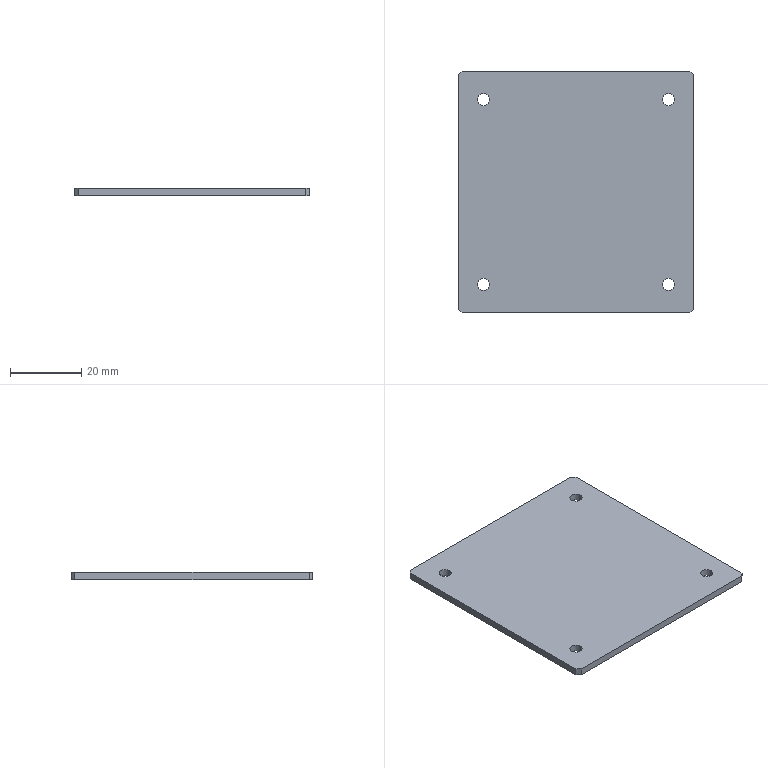Part | SolidWorks | features BaseBody 1 | 1 solid | 18 faces | box 66 x 68 x 2 mm | volume 8899 mm3 | plane 10 | cylinder 8 | commonest cylinder face diameters 3.4 x8
STEP:
#1=CARTESIAN_POINT('',(24.3,-26.,0.));
#2=VERTEX_POINT('',#1);
#3=CARTESIAN_POINT('',(27.7,-26.,0.));
#4=VERTEX_POINT('',#3);
#5=CARTESIAN_POINT('',(26.,-26.,0.));
#6=DIRECTION('',(0.,0.,1.));
#7=DIRECTION('',(1.,0.,0.));
#8=AXIS2_PLACEMENT_3D('',#5,#6,#7);
#9=CIRCLE('',#8,1.7);
#10=EDGE_CURVE('',#2,#4,#9,.T.);
#11=ORIENTED_EDGE('',*,*,#10,.F.);
#12=CARTESIAN_POINT('',(24.3,-26.,2.));
#13=VERTEX_POINT('',#12);
#14=CARTESIAN_POINT('',(24.3,-26.,2.));
#15=DIRECTION('',(0.,0.,1.));
#16=VECTOR('',#15,1000.);
#17=LINE('',#14,#16);
#18=EDGE_CURVE('',#2,#13,#17,.T.);
#19=ORIENTED_EDGE('',*,*,#18,.T.);
#20=CARTESIAN_POINT('',(27.7,-26.,2.));
#21=VERTEX_POINT('',#20);
#22=CARTESIAN_POINT('',(26.,-26.,2.));
#23=DIRECTION('',(0.,0.,-1.));
#24=DIRECTION('',(1.,0.,0.));
#25=AXIS2_PLACEMENT_3D('',#22,#23,#24);
#26=CIRCLE('',#25,1.7);
#27=EDGE_CURVE('',#21,#13,#26,.T.);
#28=ORIENTED_EDGE('',*,*,#27,.F.);
#29=CARTESIAN_POINT('',(27.7,-26.,2.));
#30=DIRECTION('',(0.,0.,1.));
#31=VECTOR('',#30,1000.);
#32=LINE('',#29,#31);
#33=EDGE_CURVE('',#4,#21,#32,.T.);
#34=ORIENTED_EDGE('',*,*,#33,.F.);
#35=EDGE_LOOP('',(#11,#19,#28,#34));
#36=FACE_OUTER_BOUND('',#35,.T.);
#37=CARTESIAN_POINT('',(26.,-26.,2.));
#38=DIRECTION('',(0.,0.,1.));
#39=DIRECTION('',(1.,0.,0.));
#40=AXIS2_PLACEMENT_3D('',#37,#38,#39);
#41=CYLINDRICAL_SURFACE('',#40,1.7);
#42=ADVANCED_FACE('',(#36),#41,.F.);
#43=CARTESIAN_POINT('',(24.3,26.,0.));
#44=VERTEX_POINT('',#43);
#45=CARTESIAN_POINT('',(27.7,26.,0.));
#46=VERTEX_POINT('',#45);
#47=CARTESIAN_POINT('',(26.,26.,0.));
#48=DIRECTION('',(0.,0.,1.));
#49=DIRECTION('',(1.,0.,0.));
#50=AXIS2_PLACEMENT_3D('',#47,#48,#49);
#51=CIRCLE('',#50,1.7);
#52=EDGE_CURVE('',#44,#46,#51,.T.);
#53=ORIENTED_EDGE('',*,*,#52,.F.);
#54=CARTESIAN_POINT('',(24.3,26.,2.));
#55=VERTEX_POINT('',#54);
#56=CARTESIAN_POINT('',(24.3,26.,2.));
#57=DIRECTION('',(0.,0.,1.));
#58=VECTOR('',#57,1000.);
#59=LINE('',#56,#58);
#60=EDGE_CURVE('',#44,#55,#59,.T.);
#61=ORIENTED_EDGE('',*,*,#60,.T.);
#62=CARTESIAN_POINT('',(27.7,26.,2.));
#63=VERTEX_POINT('',#62);
#64=CARTESIAN_POINT('',(26.,26.,2.));
#65=DIRECTION('',(0.,0.,-1.));
#66=DIRECTION('',(1.,0.,0.));
#67=AXIS2_PLACEMENT_3D('',#64,#65,#66);
#68=CIRCLE('',#67,1.7);
#69=EDGE_CURVE('',#63,#55,#68,.T.);
#70=ORIENTED_EDGE('',*,*,#69,.F.);
#71=CARTESIAN_POINT('',(27.7,26.,2.));
#72=DIRECTION('',(0.,0.,1.));
#73=VECTOR('',#72,1000.);
#74=LINE('',#71,#73);
#75=EDGE_CURVE('',#46,#63,#74,.T.);
#76=ORIENTED_EDGE('',*,*,#75,.F.);
#77=EDGE_LOOP('',(#53,#61,#70,#76));
#78=FACE_OUTER_BOUND('',#77,.T.);
#79=CARTESIAN_POINT('',(26.,26.,2.));
#80=DIRECTION('',(0.,0.,1.));
#81=DIRECTION('',(1.,0.,0.));
#82=AXIS2_PLACEMENT_3D('',#79,#80,#81);
#83=CYLINDRICAL_SURFACE('',#82,1.7);
#84=ADVANCED_FACE('',(#78),#83,.F.);
#85=CARTESIAN_POINT('',(-27.7,26.,0.));
#86=VERTEX_POINT('',#85);
#87=CARTESIAN_POINT('',(-24.3,26.,0.));
#88=VERTEX_POINT('',#87);
#89=CARTESIAN_POINT('',(-26.,26.,0.));
#90=DIRECTION('',(0.,0.,1.));
#91=DIRECTION('',(1.,0.,0.));
#92=AXIS2_PLACEMENT_3D('',#89,#90,#91);
#93=CIRCLE('',#92,1.7);
#94=EDGE_CURVE('',#86,#88,#93,.T.);
#95=ORIENTED_EDGE('',*,*,#94,.F.);
#96=CARTESIAN_POINT('',(-27.7,26.,2.));
#97=VERTEX_POINT('',#96);
#98=CARTESIAN_POINT('',(-27.7,26.,2.));
#99=DIRECTION('',(0.,0.,1.));
#100=VECTOR('',#99,1000.);
#101=LINE('',#98,#100);
#102=EDGE_CURVE('',#86,#97,#101,.T.);
#103=ORIENTED_EDGE('',*,*,#102,.T.);
#104=CARTESIAN_POINT('',(-24.3,26.,2.));
#105=VERTEX_POINT('',#104);
#106=CARTESIAN_POINT('',(-26.,26.,2.));
#107=DIRECTION('',(0.,0.,-1.));
#108=DIRECTION('',(1.,0.,0.));
#109=AXIS2_PLACEMENT_3D('',#106,#107,#108);
#110=CIRCLE('',#109,1.7);
#111=EDGE_CURVE('',#105,#97,#110,.T.);
#112=ORIENTED_EDGE('',*,*,#111,.F.);
#113=CARTESIAN_POINT('',(-24.3,26.,2.));
#114=DIRECTION('',(0.,0.,1.));
#115=VECTOR('',#114,1000.);
#116=LINE('',#113,#115);
#117=EDGE_CURVE('',#88,#105,#116,.T.);
#118=ORIENTED_EDGE('',*,*,#117,.F.);
#119=EDGE_LOOP('',(#95,#103,#112,#118));
#120=FACE_OUTER_BOUND('',#119,.T.);
#121=CARTESIAN_POINT('',(-26.,26.,2.));
#122=DIRECTION('',(0.,0.,1.));
#123=DIRECTION('',(1.,0.,0.));
#124=AXIS2_PLACEMENT_3D('',#121,#122,#123);
#125=CYLINDRICAL_SURFACE('',#124,1.7);
#126=ADVANCED_FACE('',(#120),#125,.F.);
#127=CARTESIAN_POINT('',(-27.7,-26.,0.));
#128=VERTEX_POINT('',#127);
#129=CARTESIAN_POINT('',(-24.3,-26.,0.));
#130=VERTEX_POINT('',#129);
#131=CARTESIAN_POINT('',(-26.,-26.,0.));
#132=DIRECTION('',(0.,0.,1.));
#133=DIRECTION('',(1.,0.,0.));
#134=AXIS2_PLACEMENT_3D('',#131,#132,#133);
#135=CIRCLE('',#134,1.7);
#136=EDGE_CURVE('',#128,#130,#135,.T.);
#137=ORIENTED_EDGE('',*,*,#136,.F.);
#138=CARTESIAN_POINT('',(-27.7,-26.,2.));
#139=VERTEX_POINT('',#138);
#140=CARTESIAN_POINT('',(-27.7,-26.,2.));
#141=DIRECTION('',(0.,0.,1.));
#142=VECTOR('',#141,1000.);
#143=LINE('',#140,#142);
#144=EDGE_CURVE('',#128,#139,#143,.T.);
#145=ORIENTED_EDGE('',*,*,#144,.T.);
#146=CARTESIAN_POINT('',(-24.3,-26.,2.));
#147=VERTEX_POINT('',#146);
#148=CARTESIAN_POINT('',(-26.,-26.,2.));
#149=DIRECTION('',(0.,0.,-1.));
#150=DIRECTION('',(1.,0.,0.));
#151=AXIS2_PLACEMENT_3D('',#148,#149,#150);
#152=CIRCLE('',#151,1.7);
#153=EDGE_CURVE('',#147,#139,#152,.T.);
#154=ORIENTED_EDGE('',*,*,#153,.F.);
#155=CARTESIAN_POINT('',(-24.3,-26.,2.));
#156=DIRECTION('',(0.,0.,1.));
#157=VECTOR('',#156,1000.);
#158=LINE('',#155,#157);
#159=EDGE_CURVE('',#130,#147,#158,.T.);
#160=ORIENTED_EDGE('',*,*,#159,.F.);
#161=EDGE_LOOP('',(#137,#145,#154,#160));
#162=FACE_OUTER_BOUND('',#161,.T.);
#163=CARTESIAN_POINT('',(-26.,-26.,2.));
#164=DIRECTION('',(0.,0.,1.));
#165=DIRECTION('',(1.,0.,0.));
#166=AXIS2_PLACEMENT_3D('',#163,#164,#165);
#167=CYLINDRICAL_SURFACE('',#166,1.7);
#168=ADVANCED_FACE('',(#162),#167,.F.);
#169=CARTESIAN_POINT('',(-33.,33.,2.));
#170=VERTEX_POINT('',#169);
#171=CARTESIAN_POINT('',(-33.,-33.,2.));
#172=VERTEX_POINT('',#171);
#173=CARTESIAN_POINT('',(-33.,0.,2.));
#174=DIRECTION('',(0.,-1.,0.));
#175=VECTOR('',#174,1000.);
#176=LINE('',#173,#175);
#177=EDGE_CURVE('',#170,#172,#176,.T.);
#178=ORIENTED_EDGE('',*,*,#177,.T.);
#179=CARTESIAN_POINT('',(-32.,-34.,2.));
#180=VERTEX_POINT('',#179);
#181=CARTESIAN_POINT('',(-32.,-34.,2.));
#182=DIRECTION('',(0.7071,-0.7071,0.));
#183=VECTOR('',#182,1000.);
#184=LINE('',#181,#183);
#185=EDGE_CURVE('',#172,#180,#184,.T.);
#186=ORIENTED_EDGE('',*,*,#185,.T.);
#187=CARTESIAN_POINT('',(32.,-34.,2.));
#188=VERTEX_POINT('',#187);
#189=CARTESIAN_POINT('',(0.,-34.,2.));
#190=DIRECTION('',(1.,0.,0.));
#191=VECTOR('',#190,1000.);
#192=LINE('',#189,#191);
#193=EDGE_CURVE('',#180,#188,#192,.T.);
#194=ORIENTED_EDGE('',*,*,#193,.T.);
#195=CARTESIAN_POINT('',(33.,-33.,2.));
#196=VERTEX_POINT('',#195);
#197=CARTESIAN_POINT('',(33.,-33.,2.));
#198=DIRECTION('',(0.7071,0.7071,0.));
#199=VECTOR('',#198,1000.);
#200=LINE('',#197,#199);
#201=EDGE_CURVE('',#188,#196,#200,.T.);
#202=ORIENTED_EDGE('',*,*,#201,.T.);
#203=CARTESIAN_POINT('',(33.,33.,2.));
#204=VERTEX_POINT('',#203);
#205=CARTESIAN_POINT('',(33.,0.,2.));
#206=DIRECTION('',(0.,1.,0.));
#207=VECTOR('',#206,1000.);
#208=LINE('',#205,#207);
#209=EDGE_CURVE('',#196,#204,#208,.T.);
#210=ORIENTED_EDGE('',*,*,#209,.T.);
#211=CARTESIAN_POINT('',(32.,34.,2.));
#212=VERTEX_POINT('',#211);
#213=CARTESIAN_POINT('',(32.,34.,2.));
#214=DIRECTION('',(-0.7071,0.7071,0.));
#215=VECTOR('',#214,1000.);
#216=LINE('',#213,#215);
#217=EDGE_CURVE('',#204,#212,#216,.T.);
#218=ORIENTED_EDGE('',*,*,#217,.T.);
#219=CARTESIAN_POINT('',(-32.,34.,2.));
#220=VERTEX_POINT('',#219);
#221=CARTESIAN_POINT('',(0.,34.,2.));
#222=DIRECTION('',(-1.,0.,0.));
#223=VECTOR('',#222,1000.);
#224=LINE('',#221,#223);
#225=EDGE_CURVE('',#212,#220,#224,.T.);
#226=ORIENTED_EDGE('',*,*,#225,.T.);
#227=CARTESIAN_POINT('',(-33.,33.,2.));
#228=DIRECTION('',(-0.7071,-0.7071,0.));
#229=VECTOR('',#228,1000.);
#230=LINE('',#227,#229);
#231=EDGE_CURVE('',#220,#170,#230,.T.);
#232=ORIENTED_EDGE('',*,*,#231,.T.);
#233=EDGE_LOOP('',(#178,#186,#194,#202,#210,#218,#226,#232));
#234=FACE_OUTER_BOUND('',#233,.T.);
#235=ORIENTED_EDGE('',*,*,#27,.T.);
#236=CARTESIAN_POINT('',(26.,-26.,2.));
#237=DIRECTION('',(0.,0.,-1.));
#238=DIRECTION('',(1.,0.,0.));
#239=AXIS2_PLACEMENT_3D('',#236,#237,#238);
#240=CIRCLE('',#239,1.7);
#241=EDGE_CURVE('',#13,#21,#240,.T.);
#242=ORIENTED_EDGE('',*,*,#241,.T.);
#243=EDGE_LOOP('',(#235,#242));
#244=FACE_BOUND('',#243,.T.);
#245=ORIENTED_EDGE('',*,*,#69,.T.);
#246=CARTESIAN_POINT('',(26.,26.,2.));
#247=DIRECTION('',(0.,0.,-1.));
#248=DIRECTION('',(1.,0.,0.));
#249=AXIS2_PLACEMENT_3D('',#246,#247,#248);
#250=CIRCLE('',#249,1.7);
#251=EDGE_CURVE('',#55,#63,#250,.T.);
#252=ORIENTED_EDGE('',*,*,#251,.T.);
#253=EDGE_LOOP('',(#245,#252));
#254=FACE_BOUND('',#253,.T.);
#255=ORIENTED_EDGE('',*,*,#111,.T.);
#256=CARTESIAN_POINT('',(-26.,26.,2.));
#257=DIRECTION('',(0.,0.,-1.));
#258=DIRECTION('',(1.,0.,0.));
#259=AXIS2_PLACEMENT_3D('',#256,#257,#258);
#260=CIRCLE('',#259,1.7);
#261=EDGE_CURVE('',#97,#105,#260,.T.);
#262=ORIENTED_EDGE('',*,*,#261,.T.);
#263=EDGE_LOOP('',(#255,#262));
#264=FACE_BOUND('',#263,.T.);
#265=ORIENTED_EDGE('',*,*,#153,.T.);
#266=CARTESIAN_POINT('',(-26.,-26.,2.));
#267=DIRECTION('',(0.,0.,-1.));
#268=DIRECTION('',(1.,0.,0.));
#269=AXIS2_PLACEMENT_3D('',#266,#267,#268);
#270=CIRCLE('',#269,1.7);
#271=EDGE_CURVE('',#139,#147,#270,.T.);
#272=ORIENTED_EDGE('',*,*,#271,.T.);
#273=EDGE_LOOP('',(#265,#272));
#274=FACE_BOUND('',#273,.T.);
#275=CARTESIAN_POINT('',(0.,0.,2.));
#276=DIRECTION('',(0.,0.,1.));
#277=DIRECTION('',(1.,0.,0.));
#278=AXIS2_PLACEMENT_3D('',#275,#276,#277);
#279=PLANE('',#278);
#280=ADVANCED_FACE('',(#234,#244,#254,#264,#274),#279,.T.);
#281=CARTESIAN_POINT('',(-33.,-33.,0.));
#282=VERTEX_POINT('',#281);
#283=CARTESIAN_POINT('',(-33.,-33.,2.));
#284=DIRECTION('',(0.,0.,-1.));
#285=VECTOR('',#284,1000.);
#286=LINE('',#283,#285);
#287=EDGE_CURVE('',#172,#282,#286,.T.);
#288=ORIENTED_EDGE('',*,*,#287,.F.);
#289=ORIENTED_EDGE('',*,*,#177,.F.);
#290=CARTESIAN_POINT('',(-33.,33.,0.));
#291=VERTEX_POINT('',#290);
#292=CARTESIAN_POINT('',(-33.,33.,2.));
#293=DIRECTION('',(0.,0.,1.));
#294=VECTOR('',#293,1000.);
#295=LINE('',#292,#294);
#296=EDGE_CURVE('',#291,#170,#295,.T.);
#297=ORIENTED_EDGE('',*,*,#296,.F.);
#298=CARTESIAN_POINT('',(-33.,34.,0.));
#299=DIRECTION('',(0.,1.,0.));
#300=VECTOR('',#299,1000.);
#301=LINE('',#298,#300);
#302=EDGE_CURVE('',#282,#291,#301,.T.);
#303=ORIENTED_EDGE('',*,*,#302,.F.);
#304=EDGE_LOOP('',(#288,#289,#297,#303));
#305=FACE_OUTER_BOUND('',#304,.T.);
#306=CARTESIAN_POINT('',(-33.,34.,2.));
#307=DIRECTION('',(1.,0.,0.));
#308=DIRECTION('',(0.,1.,0.));
#309=AXIS2_PLACEMENT_3D('',#306,#307,#308);
#310=PLANE('',#309);
#311=ADVANCED_FACE('',(#305),#310,.F.);
#312=CARTESIAN_POINT('',(32.,34.,0.));
#313=VERTEX_POINT('',#312);
#314=CARTESIAN_POINT('',(32.,34.,2.));
#315=DIRECTION('',(0.,0.,1.));
#316=VECTOR('',#315,1000.);
#317=LINE('',#314,#316);
#318=EDGE_CURVE('',#313,#212,#317,.T.);
#319=ORIENTED_EDGE('',*,*,#318,.F.);
#320=CARTESIAN_POINT('',(-32.,34.,0.));
#321=VERTEX_POINT('',#320);
#322=CARTESIAN_POINT('',(-33.,34.,0.));
#323=DIRECTION('',(1.,0.,0.));
#324=VECTOR('',#323,1000.);
#325=LINE('',#322,#324);
#326=EDGE_CURVE('',#321,#313,#325,.T.);
#327=ORIENTED_EDGE('',*,*,#326,.F.);
#328=CARTESIAN_POINT('',(-32.,34.,2.));
#329=DIRECTION('',(0.,0.,-1.));
#330=VECTOR('',#329,1000.);
#331=LINE('',#328,#330);
#332=EDGE_CURVE('',#220,#321,#331,.T.);
#333=ORIENTED_EDGE('',*,*,#332,.F.);
#334=ORIENTED_EDGE('',*,*,#225,.F.);
#335=EDGE_LOOP('',(#319,#327,#333,#334));
#336=FACE_OUTER_BOUND('',#335,.T.);
#337=CARTESIAN_POINT('',(-33.,34.,2.));
#338=DIRECTION('',(0.,-1.,0.));
#339=DIRECTION('',(1.,0.,0.));
#340=AXIS2_PLACEMENT_3D('',#337,#338,#339);
#341=PLANE('',#340);
#342=ADVANCED_FACE('',(#336),#341,.F.);
#343=CARTESIAN_POINT('',(33.,-33.,0.));
#344=VERTEX_POINT('',#343);
#345=CARTESIAN_POINT('',(33.,-33.,2.));
#346=DIRECTION('',(0.,0.,1.));
#347=VECTOR('',#346,1000.);
#348=LINE('',#345,#347);
#349=EDGE_CURVE('',#344,#196,#348,.T.);
#350=ORIENTED_EDGE('',*,*,#349,.F.);
#351=CARTESIAN_POINT('',(33.,33.,0.));
#352=VERTEX_POINT('',#351);
#353=CARTESIAN_POINT('',(33.,34.,0.));
#354=DIRECTION('',(0.,-1.,0.));
#355=VECTOR('',#354,1000.);
#356=LINE('',#353,#355);
#357=EDGE_CURVE('',#352,#344,#356,.T.);
#358=ORIENTED_EDGE('',*,*,#357,.F.);
#359=CARTESIAN_POINT('',(33.,33.,2.));
#360=DIRECTION('',(0.,0.,-1.));
#361=VECTOR('',#360,1000.);
#362=LINE('',#359,#361);
#363=EDGE_CURVE('',#204,#352,#362,.T.);
#364=ORIENTED_EDGE('',*,*,#363,.F.);
#365=ORIENTED_EDGE('',*,*,#209,.F.);
#366=EDGE_LOOP('',(#350,#358,#364,#365));
#367=FACE_OUTER_BOUND('',#366,.T.);
#368=CARTESIAN_POINT('',(33.,34.,2.));
#369=DIRECTION('',(-1.,0.,0.));
#370=DIRECTION('',(0.,-1.,0.));
#371=AXIS2_PLACEMENT_3D('',#368,#369,#370);
#372=PLANE('',#371);
#373=ADVANCED_FACE('',(#367),#372,.F.);
#374=CARTESIAN_POINT('',(32.,-34.,0.));
#375=VERTEX_POINT('',#374);
#376=CARTESIAN_POINT('',(32.,-34.,2.));
#377=DIRECTION('',(0.,0.,-1.));
#378=VECTOR('',#377,1000.);
#379=LINE('',#376,#378);
#380=EDGE_CURVE('',#188,#375,#379,.T.);
#381=ORIENTED_EDGE('',*,*,#380,.F.);
#382=ORIENTED_EDGE('',*,*,#193,.F.);
#383=CARTESIAN_POINT('',(-32.,-34.,0.));
#384=VERTEX_POINT('',#383);
#385=CARTESIAN_POINT('',(-32.,-34.,2.));
#386=DIRECTION('',(0.,0.,1.));
#387=VECTOR('',#386,1000.);
#388=LINE('',#385,#387);
#389=EDGE_CURVE('',#384,#180,#388,.T.);
#390=ORIENTED_EDGE('',*,*,#389,.F.);
#391=CARTESIAN_POINT('',(-33.,-34.,0.));
#392=DIRECTION('',(-1.,0.,0.));
#393=VECTOR('',#392,1000.);
#394=LINE('',#391,#393);
#395=EDGE_CURVE('',#375,#384,#394,.T.);
#396=ORIENTED_EDGE('',*,*,#395,.F.);
#397=EDGE_LOOP('',(#381,#382,#390,#396));
#398=FACE_OUTER_BOUND('',#397,.T.);
#399=CARTESIAN_POINT('',(-33.,-34.,2.));
#400=DIRECTION('',(0.,1.,0.));
#401=DIRECTION('',(-1.,0.,0.));
#402=AXIS2_PLACEMENT_3D('',#399,#400,#401);
#403=PLANE('',#402);
#404=ADVANCED_FACE('',(#398),#403,.F.);
#405=ORIENTED_EDGE('',*,*,#18,.F.);
#406=CARTESIAN_POINT('',(26.,-26.,0.));
#407=DIRECTION('',(0.,0.,1.));
#408=DIRECTION('',(1.,0.,0.));
#409=AXIS2_PLACEMENT_3D('',#406,#407,#408);
#410=CIRCLE('',#409,1.7);
#411=EDGE_CURVE('',#4,#2,#410,.T.);
#412=ORIENTED_EDGE('',*,*,#411,.F.);
#413=ORIENTED_EDGE('',*,*,#33,.T.);
#414=ORIENTED_EDGE('',*,*,#241,.F.);
#415=EDGE_LOOP('',(#405,#412,#413,#414));
#416=FACE_OUTER_BOUND('',#415,.T.);
#417=CARTESIAN_POINT('',(26.,-26.,2.));
#418=DIRECTION('',(0.,0.,1.));
#419=DIRECTION('',(1.,0.,0.));
#420=AXIS2_PLACEMENT_3D('',#417,#418,#419);
#421=CYLINDRICAL_SURFACE('',#420,1.7);
#422=ADVANCED_FACE('',(#416),#421,.F.);
#423=ORIENTED_EDGE('',*,*,#60,.F.);
#424=CARTESIAN_POINT('',(26.,26.,0.));
#425=DIRECTION('',(0.,0.,1.));
#426=DIRECTION('',(1.,0.,0.));
#427=AXIS2_PLACEMENT_3D('',#424,#425,#426);
#428=CIRCLE('',#427,1.7);
#429=EDGE_CURVE('',#46,#44,#428,.T.);
#430=ORIENTED_EDGE('',*,*,#429,.F.);
#431=ORIENTED_EDGE('',*,*,#75,.T.);
#432=ORIENTED_EDGE('',*,*,#251,.F.);
#433=EDGE_LOOP('',(#423,#430,#431,#432));
#434=FACE_OUTER_BOUND('',#433,.T.);
#435=CARTESIAN_POINT('',(26.,26.,2.));
#436=DIRECTION('',(0.,0.,1.));
#437=DIRECTION('',(1.,0.,0.));
#438=AXIS2_PLACEMENT_3D('',#435,#436,#437);
#439=CYLINDRICAL_SURFACE('',#438,1.7);
#440=ADVANCED_FACE('',(#434),#439,.F.);
#441=ORIENTED_EDGE('',*,*,#102,.F.);
#442=CARTESIAN_POINT('',(-26.,26.,0.));
#443=DIRECTION('',(0.,0.,1.));
#444=DIRECTION('',(1.,0.,0.));
#445=AXIS2_PLACEMENT_3D('',#442,#443,#444);
#446=CIRCLE('',#445,1.7);
#447=EDGE_CURVE('',#88,#86,#446,.T.);
#448=ORIENTED_EDGE('',*,*,#447,.F.);
#449=ORIENTED_EDGE('',*,*,#117,.T.);
#450=ORIENTED_EDGE('',*,*,#261,.F.);
#451=EDGE_LOOP('',(#441,#448,#449,#450));
#452=FACE_OUTER_BOUND('',#451,.T.);
#453=CARTESIAN_POINT('',(-26.,26.,2.));
#454=DIRECTION('',(0.,0.,1.));
#455=DIRECTION('',(1.,0.,0.));
#456=AXIS2_PLACEMENT_3D('',#453,#454,#455);
#457=CYLINDRICAL_SURFACE('',#456,1.7);
#458=ADVANCED_FACE('',(#452),#457,.F.);
#459=ORIENTED_EDGE('',*,*,#144,.F.);
#460=CARTESIAN_POINT('',(-26.,-26.,0.));
#461=DIRECTION('',(0.,0.,1.));
#462=DIRECTION('',(1.,0.,0.));
#463=AXIS2_PLACEMENT_3D('',#460,#461,#462);
#464=CIRCLE('',#463,1.7);
#465=EDGE_CURVE('',#130,#128,#464,.T.);
#466=ORIENTED_EDGE('',*,*,#465,.F.);
#467=ORIENTED_EDGE('',*,*,#159,.T.);
#468=ORIENTED_EDGE('',*,*,#271,.F.);
#469=EDGE_LOOP('',(#459,#466,#467,#468));
#470=FACE_OUTER_BOUND('',#469,.T.);
#471=CARTESIAN_POINT('',(-26.,-26.,2.));
#472=DIRECTION('',(0.,0.,1.));
#473=DIRECTION('',(1.,0.,0.));
#474=AXIS2_PLACEMENT_3D('',#471,#472,#473);
#475=CYLINDRICAL_SURFACE('',#474,1.7);
#476=ADVANCED_FACE('',(#470),#475,.F.);
#477=CARTESIAN_POINT('',(32.,-34.,0.));
#478=DIRECTION('',(0.7071,0.7071,0.));
#479=VECTOR('',#478,1000.);
#480=LINE('',#477,#479);
#481=EDGE_CURVE('',#375,#344,#480,.T.);
#482=ORIENTED_EDGE('',*,*,#481,.F.);
#483=ORIENTED_EDGE('',*,*,#395,.T.);
#484=CARTESIAN_POINT('',(-33.,-33.,0.));
#485=DIRECTION('',(0.7071,-0.7071,0.));
#486=VECTOR('',#485,1000.);
#487=LINE('',#484,#486);
#488=EDGE_CURVE('',#282,#384,#487,.T.);
#489=ORIENTED_EDGE('',*,*,#488,.F.);
#490=ORIENTED_EDGE('',*,*,#302,.T.);
#491=CARTESIAN_POINT('',(-32.,34.,0.));
#492=DIRECTION('',(-0.7071,-0.7071,0.));
#493=VECTOR('',#492,1000.);
#494=LINE('',#491,#493);
#495=EDGE_CURVE('',#321,#291,#494,.T.);
#496=ORIENTED_EDGE('',*,*,#495,.F.);
#497=ORIENTED_EDGE('',*,*,#326,.T.);
#498=CARTESIAN_POINT('',(33.,33.,0.));
#499=DIRECTION('',(-0.7071,0.7071,0.));
#500=VECTOR('',#499,1000.);
#501=LINE('',#498,#500);
#502=EDGE_CURVE('',#352,#313,#501,.T.);
#503=ORIENTED_EDGE('',*,*,#502,.F.);
#504=ORIENTED_EDGE('',*,*,#357,.T.);
#505=EDGE_LOOP('',(#482,#483,#489,#490,#496,#497,#503,#504));
#506=FACE_OUTER_BOUND('',#505,.T.);
#507=ORIENTED_EDGE('',*,*,#411,.T.);
#508=ORIENTED_EDGE('',*,*,#10,.T.);
#509=EDGE_LOOP('',(#507,#508));
#510=FACE_BOUND('',#509,.T.);
#511=ORIENTED_EDGE('',*,*,#429,.T.);
#512=ORIENTED_EDGE('',*,*,#52,.T.);
#513=EDGE_LOOP('',(#511,#512));
#514=FACE_BOUND('',#513,.T.);
#515=ORIENTED_EDGE('',*,*,#447,.T.);
#516=ORIENTED_EDGE('',*,*,#94,.T.);
#517=EDGE_LOOP('',(#515,#516));
#518=FACE_BOUND('',#517,.T.);
#519=ORIENTED_EDGE('',*,*,#465,.T.);
#520=ORIENTED_EDGE('',*,*,#136,.T.);
#521=EDGE_LOOP('',(#519,#520));
#522=FACE_BOUND('',#521,.T.);
#523=CARTESIAN_POINT('',(0.,0.,0.));
#524=DIRECTION('',(0.,0.,1.));
#525=DIRECTION('',(1.,0.,0.));
#526=AXIS2_PLACEMENT_3D('',#523,#524,#525);
#527=PLANE('',#526);
#528=ADVANCED_FACE('',(#506,#510,#514,#518,#522),#527,.F.);
#529=ORIENTED_EDGE('',*,*,#287,.T.);
#530=ORIENTED_EDGE('',*,*,#488,.T.);
#531=ORIENTED_EDGE('',*,*,#389,.T.);
#532=ORIENTED_EDGE('',*,*,#185,.F.);
#533=EDGE_LOOP('',(#529,#530,#531,#532));
#534=FACE_OUTER_BOUND('',#533,.T.);
#535=CARTESIAN_POINT('',(-32.,-34.,2.));
#536=DIRECTION('',(0.7071,0.7071,0.));
#537=DIRECTION('',(-0.7071,0.7071,0.));
#538=AXIS2_PLACEMENT_3D('',#535,#536,#537);
#539=PLANE('',#538);
#540=ADVANCED_FACE('',(#534),#539,.F.);
#541=ORIENTED_EDGE('',*,*,#332,.T.);
#542=ORIENTED_EDGE('',*,*,#495,.T.);
#543=ORIENTED_EDGE('',*,*,#296,.T.);
#544=ORIENTED_EDGE('',*,*,#231,.F.);
#545=EDGE_LOOP('',(#541,#542,#543,#544));
#546=FACE_OUTER_BOUND('',#545,.T.);
#547=CARTESIAN_POINT('',(-33.,33.,2.));
#548=DIRECTION('',(0.7071,-0.7071,0.));
#549=DIRECTION('',(0.7071,0.7071,0.));
#550=AXIS2_PLACEMENT_3D('',#547,#548,#549);
#551=PLANE('',#550);
#552=ADVANCED_FACE('',(#546),#551,.F.);
#553=ORIENTED_EDGE('',*,*,#363,.T.);
#554=ORIENTED_EDGE('',*,*,#502,.T.);
#555=ORIENTED_EDGE('',*,*,#318,.T.);
#556=ORIENTED_EDGE('',*,*,#217,.F.);
#557=EDGE_LOOP('',(#553,#554,#555,#556));
#558=FACE_OUTER_BOUND('',#557,.T.);
#559=CARTESIAN_POINT('',(32.,34.,2.));
#560=DIRECTION('',(-0.7071,-0.7071,0.));
#561=DIRECTION('',(0.7071,-0.7071,0.));
#562=AXIS2_PLACEMENT_3D('',#559,#560,#561);
#563=PLANE('',#562);
#564=ADVANCED_FACE('',(#558),#563,.F.);
#565=ORIENTED_EDGE('',*,*,#380,.T.);
#566=ORIENTED_EDGE('',*,*,#481,.T.);
#567=ORIENTED_EDGE('',*,*,#349,.T.);
#568=ORIENTED_EDGE('',*,*,#201,.F.);
#569=EDGE_LOOP('',(#565,#566,#567,#568));
#570=FACE_OUTER_BOUND('',#569,.T.);
#571=CARTESIAN_POINT('',(33.,-33.,2.));
#572=DIRECTION('',(-0.7071,0.7071,0.));
#573=DIRECTION('',(-0.7071,-0.7071,0.));
#574=AXIS2_PLACEMENT_3D('',#571,#572,#573);
#575=PLANE('',#574);
#576=ADVANCED_FACE('',(#570),#575,.F.);
#577=CLOSED_SHELL('',(#42,#84,#126,#168,#280,#311,#342,#373,#404,#422,#440,#458,#476,#528,#540,#552,#564,#576));
#578=MANIFOLD_SOLID_BREP('',#577);
#579=CARTESIAN_POINT('',(0.,0.,0.));
#580=DIRECTION('',(0.,0.,1.));
#581=DIRECTION('',(1.,0.,0.));
#582=AXIS2_PLACEMENT_3D('',#579,#580,#581);
#583=(LENGTH_UNIT()NAMED_UNIT(*)SI_UNIT(.MILLI.,.METRE.));
#584=UNCERTAINTY_MEASURE_WITH_UNIT(LENGTH_MEASURE(0.00001),#583,'','');
#585=(NAMED_UNIT(*)PLANE_ANGLE_UNIT()SI_UNIT($,.RADIAN.));
#586=(NAMED_UNIT(*)SI_UNIT($,.STERADIAN.)SOLID_ANGLE_UNIT());
#587=(GEOMETRIC_REPRESENTATION_CONTEXT(3)GLOBAL_UNCERTAINTY_ASSIGNED_CONTEXT((#584))GLOBAL_UNIT_ASSIGNED_CONTEXT((#583,#585,#586))REPRESENTATION_CONTEXT('',''));
#588=ADVANCED_BREP_SHAPE_REPRESENTATION('',(#578,#582),#587);